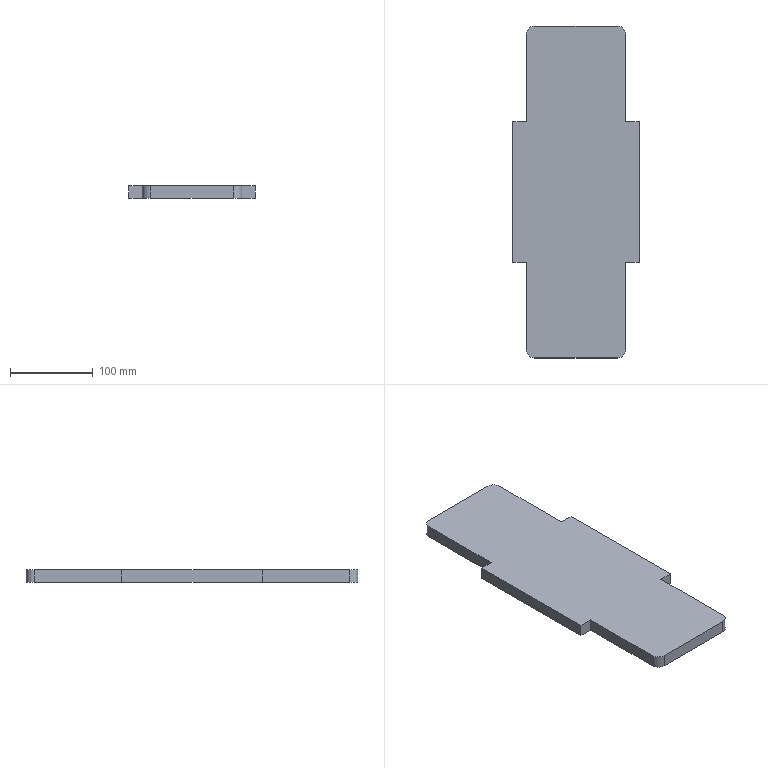Part | STEP file | adapter plate^three-axis module | 1 solid | 18 faces | box 152 x 400 x 15 mm | volume 799832 mm3 | plane 14 | cylinder 4 | commonest cylinder face diameters 20 x4
STEP:
#1=CARTESIAN_POINT('',(-60.,190.,15.));
#2=VERTEX_POINT('',#1);
#3=CARTESIAN_POINT('',(-60.,84.5,15.));
#4=VERTEX_POINT('',#3);
#5=CARTESIAN_POINT('',(-60.,0.,15.));
#6=DIRECTION('',(0.,-1.,0.));
#7=VECTOR('',#6,1000.);
#8=LINE('',#5,#7);
#9=EDGE_CURVE('',#2,#4,#8,.T.);
#10=ORIENTED_EDGE('',*,*,#9,.T.);
#11=CARTESIAN_POINT('',(-76.,84.5,15.));
#12=VERTEX_POINT('',#11);
#13=CARTESIAN_POINT('',(0.,84.5,15.));
#14=DIRECTION('',(-1.,0.,0.));
#15=VECTOR('',#14,1000.);
#16=LINE('',#13,#15);
#17=EDGE_CURVE('',#4,#12,#16,.T.);
#18=ORIENTED_EDGE('',*,*,#17,.T.);
#19=CARTESIAN_POINT('',(-76.,-84.5,15.));
#20=VERTEX_POINT('',#19);
#21=CARTESIAN_POINT('',(-76.,0.,15.));
#22=DIRECTION('',(0.,-1.,0.));
#23=VECTOR('',#22,1000.);
#24=LINE('',#21,#23);
#25=EDGE_CURVE('',#12,#20,#24,.T.);
#26=ORIENTED_EDGE('',*,*,#25,.T.);
#27=CARTESIAN_POINT('',(-60.,-84.5,15.));
#28=VERTEX_POINT('',#27);
#29=CARTESIAN_POINT('',(0.,-84.5,15.));
#30=DIRECTION('',(1.,0.,0.));
#31=VECTOR('',#30,1000.);
#32=LINE('',#29,#31);
#33=EDGE_CURVE('',#20,#28,#32,.T.);
#34=ORIENTED_EDGE('',*,*,#33,.T.);
#35=CARTESIAN_POINT('',(-60.,-190.,15.));
#36=VERTEX_POINT('',#35);
#37=CARTESIAN_POINT('',(-60.,0.,15.));
#38=DIRECTION('',(0.,-1.,0.));
#39=VECTOR('',#38,1000.);
#40=LINE('',#37,#39);
#41=EDGE_CURVE('',#28,#36,#40,.T.);
#42=ORIENTED_EDGE('',*,*,#41,.T.);
#43=CARTESIAN_POINT('',(-50.,-200.,15.));
#44=VERTEX_POINT('',#43);
#45=CARTESIAN_POINT('',(-50.,-190.,15.));
#46=DIRECTION('',(0.,0.,1.));
#47=DIRECTION('',(1.,0.,0.));
#48=AXIS2_PLACEMENT_3D('',#45,#46,#47);
#49=CIRCLE('',#48,10.);
#50=EDGE_CURVE('',#36,#44,#49,.T.);
#51=ORIENTED_EDGE('',*,*,#50,.T.);
#52=CARTESIAN_POINT('',(50.,-200.,15.));
#53=VERTEX_POINT('',#52);
#54=CARTESIAN_POINT('',(0.,-200.,15.));
#55=DIRECTION('',(1.,0.,0.));
#56=VECTOR('',#55,1000.);
#57=LINE('',#54,#56);
#58=EDGE_CURVE('',#44,#53,#57,.T.);
#59=ORIENTED_EDGE('',*,*,#58,.T.);
#60=CARTESIAN_POINT('',(60.,-190.,15.));
#61=VERTEX_POINT('',#60);
#62=CARTESIAN_POINT('',(50.,-190.,15.));
#63=DIRECTION('',(0.,0.,1.));
#64=DIRECTION('',(1.,0.,0.));
#65=AXIS2_PLACEMENT_3D('',#62,#63,#64);
#66=CIRCLE('',#65,10.);
#67=EDGE_CURVE('',#53,#61,#66,.T.);
#68=ORIENTED_EDGE('',*,*,#67,.T.);
#69=CARTESIAN_POINT('',(60.,-84.5,15.));
#70=VERTEX_POINT('',#69);
#71=CARTESIAN_POINT('',(60.,0.,15.));
#72=DIRECTION('',(0.,1.,0.));
#73=VECTOR('',#72,1000.);
#74=LINE('',#71,#73);
#75=EDGE_CURVE('',#61,#70,#74,.T.);
#76=ORIENTED_EDGE('',*,*,#75,.T.);
#77=CARTESIAN_POINT('',(76.,-84.5,15.));
#78=VERTEX_POINT('',#77);
#79=CARTESIAN_POINT('',(0.,-84.5,15.));
#80=DIRECTION('',(1.,0.,0.));
#81=VECTOR('',#80,1000.);
#82=LINE('',#79,#81);
#83=EDGE_CURVE('',#70,#78,#82,.T.);
#84=ORIENTED_EDGE('',*,*,#83,.T.);
#85=CARTESIAN_POINT('',(76.,84.5,15.));
#86=VERTEX_POINT('',#85);
#87=CARTESIAN_POINT('',(76.,0.,15.));
#88=DIRECTION('',(0.,1.,0.));
#89=VECTOR('',#88,1000.);
#90=LINE('',#87,#89);
#91=EDGE_CURVE('',#78,#86,#90,.T.);
#92=ORIENTED_EDGE('',*,*,#91,.T.);
#93=CARTESIAN_POINT('',(60.,84.5,15.));
#94=VERTEX_POINT('',#93);
#95=CARTESIAN_POINT('',(0.,84.5,15.));
#96=DIRECTION('',(-1.,0.,0.));
#97=VECTOR('',#96,1000.);
#98=LINE('',#95,#97);
#99=EDGE_CURVE('',#86,#94,#98,.T.);
#100=ORIENTED_EDGE('',*,*,#99,.T.);
#101=CARTESIAN_POINT('',(60.,190.,15.));
#102=VERTEX_POINT('',#101);
#103=CARTESIAN_POINT('',(60.,0.,15.));
#104=DIRECTION('',(0.,1.,0.));
#105=VECTOR('',#104,1000.);
#106=LINE('',#103,#105);
#107=EDGE_CURVE('',#94,#102,#106,.T.);
#108=ORIENTED_EDGE('',*,*,#107,.T.);
#109=CARTESIAN_POINT('',(50.,200.,15.));
#110=VERTEX_POINT('',#109);
#111=CARTESIAN_POINT('',(50.,190.,15.));
#112=DIRECTION('',(0.,0.,1.));
#113=DIRECTION('',(1.,0.,0.));
#114=AXIS2_PLACEMENT_3D('',#111,#112,#113);
#115=CIRCLE('',#114,10.);
#116=EDGE_CURVE('',#102,#110,#115,.T.);
#117=ORIENTED_EDGE('',*,*,#116,.T.);
#118=CARTESIAN_POINT('',(-50.,200.,15.));
#119=VERTEX_POINT('',#118);
#120=CARTESIAN_POINT('',(0.,200.,15.));
#121=DIRECTION('',(-1.,0.,0.));
#122=VECTOR('',#121,1000.);
#123=LINE('',#120,#122);
#124=EDGE_CURVE('',#110,#119,#123,.T.);
#125=ORIENTED_EDGE('',*,*,#124,.T.);
#126=CARTESIAN_POINT('',(-50.,190.,15.));
#127=DIRECTION('',(0.,0.,1.));
#128=DIRECTION('',(1.,0.,0.));
#129=AXIS2_PLACEMENT_3D('',#126,#127,#128);
#130=CIRCLE('',#129,10.);
#131=EDGE_CURVE('',#119,#2,#130,.T.);
#132=ORIENTED_EDGE('',*,*,#131,.T.);
#133=EDGE_LOOP('',(#10,#18,#26,#34,#42,#51,#59,#68,#76,#84,#92,#100,#108,#117,#125,#132));
#134=FACE_OUTER_BOUND('',#133,.T.);
#135=CARTESIAN_POINT('',(0.,0.,15.));
#136=DIRECTION('',(0.,0.,1.));
#137=DIRECTION('',(1.,0.,0.));
#138=AXIS2_PLACEMENT_3D('',#135,#136,#137);
#139=PLANE('',#138);
#140=ADVANCED_FACE('',(#134),#139,.T.);
#141=CARTESIAN_POINT('',(-76.,84.5,0.));
#142=VERTEX_POINT('',#141);
#143=CARTESIAN_POINT('',(-76.,84.5,15.));
#144=DIRECTION('',(0.,0.,-1.));
#145=VECTOR('',#144,1000.);
#146=LINE('',#143,#145);
#147=EDGE_CURVE('',#12,#142,#146,.T.);
#148=ORIENTED_EDGE('',*,*,#147,.F.);
#149=ORIENTED_EDGE('',*,*,#17,.F.);
#150=CARTESIAN_POINT('',(-60.,84.5,0.));
#151=VERTEX_POINT('',#150);
#152=CARTESIAN_POINT('',(-60.,84.5,15.));
#153=DIRECTION('',(0.,0.,1.));
#154=VECTOR('',#153,1000.);
#155=LINE('',#152,#154);
#156=EDGE_CURVE('',#151,#4,#155,.T.);
#157=ORIENTED_EDGE('',*,*,#156,.F.);
#158=CARTESIAN_POINT('',(-76.,84.5,0.));
#159=DIRECTION('',(1.,0.,0.));
#160=VECTOR('',#159,1000.);
#161=LINE('',#158,#160);
#162=EDGE_CURVE('',#142,#151,#161,.T.);
#163=ORIENTED_EDGE('',*,*,#162,.F.);
#164=EDGE_LOOP('',(#148,#149,#157,#163));
#165=FACE_OUTER_BOUND('',#164,.T.);
#166=CARTESIAN_POINT('',(-76.,84.5,15.));
#167=DIRECTION('',(0.,-1.,0.));
#168=DIRECTION('',(0.,0.,-1.));
#169=AXIS2_PLACEMENT_3D('',#166,#167,#168);
#170=PLANE('',#169);
#171=ADVANCED_FACE('',(#165),#170,.F.);
#172=CARTESIAN_POINT('',(-60.,190.,0.));
#173=VERTEX_POINT('',#172);
#174=CARTESIAN_POINT('',(-60.,200.,0.));
#175=DIRECTION('',(0.,-1.,0.));
#176=VECTOR('',#175,1000.);
#177=LINE('',#174,#176);
#178=EDGE_CURVE('',#173,#151,#177,.T.);
#179=ORIENTED_EDGE('',*,*,#178,.T.);
#180=ORIENTED_EDGE('',*,*,#156,.T.);
#181=ORIENTED_EDGE('',*,*,#9,.F.);
#182=CARTESIAN_POINT('',(-60.,190.,-417.612));
#183=DIRECTION('',(0.,0.,-1.));
#184=VECTOR('',#183,1000.);
#185=LINE('',#182,#184);
#186=EDGE_CURVE('',#2,#173,#185,.T.);
#187=ORIENTED_EDGE('',*,*,#186,.T.);
#188=EDGE_LOOP('',(#179,#180,#181,#187));
#189=FACE_OUTER_BOUND('',#188,.T.);
#190=CARTESIAN_POINT('',(-60.,200.,-417.612));
#191=DIRECTION('',(-1.,0.,0.));
#192=DIRECTION('',(0.,-1.,0.));
#193=AXIS2_PLACEMENT_3D('',#190,#191,#192);
#194=PLANE('',#193);
#195=ADVANCED_FACE('',(#189),#194,.T.);
#196=ORIENTED_EDGE('',*,*,#131,.F.);
#197=CARTESIAN_POINT('',(-50.,200.,0.));
#198=VERTEX_POINT('',#197);
#199=CARTESIAN_POINT('',(-50.,200.,-417.612));
#200=DIRECTION('',(0.,0.,-1.));
#201=VECTOR('',#200,1000.);
#202=LINE('',#199,#201);
#203=EDGE_CURVE('',#119,#198,#202,.T.);
#204=ORIENTED_EDGE('',*,*,#203,.T.);
#205=CARTESIAN_POINT('',(-50.,190.,0.));
#206=DIRECTION('',(0.,0.,1.));
#207=DIRECTION('',(1.,0.,0.));
#208=AXIS2_PLACEMENT_3D('',#205,#206,#207);
#209=CIRCLE('',#208,10.);
#210=EDGE_CURVE('',#198,#173,#209,.T.);
#211=ORIENTED_EDGE('',*,*,#210,.T.);
#212=ORIENTED_EDGE('',*,*,#186,.F.);
#213=EDGE_LOOP('',(#196,#204,#211,#212));
#214=FACE_OUTER_BOUND('',#213,.T.);
#215=CARTESIAN_POINT('',(-50.,190.,-417.612));
#216=DIRECTION('',(0.,0.,1.));
#217=DIRECTION('',(1.,0.,0.));
#218=AXIS2_PLACEMENT_3D('',#215,#216,#217);
#219=CYLINDRICAL_SURFACE('',#218,10.);
#220=ADVANCED_FACE('',(#214),#219,.T.);
#221=CARTESIAN_POINT('',(50.,200.,0.));
#222=VERTEX_POINT('',#221);
#223=CARTESIAN_POINT('',(-60.,200.,0.));
#224=DIRECTION('',(-1.,0.,0.));
#225=VECTOR('',#224,1000.);
#226=LINE('',#223,#225);
#227=EDGE_CURVE('',#222,#198,#226,.T.);
#228=ORIENTED_EDGE('',*,*,#227,.T.);
#229=ORIENTED_EDGE('',*,*,#203,.F.);
#230=ORIENTED_EDGE('',*,*,#124,.F.);
#231=CARTESIAN_POINT('',(50.,200.,-417.612));
#232=DIRECTION('',(0.,0.,-1.));
#233=VECTOR('',#232,1000.);
#234=LINE('',#231,#233);
#235=EDGE_CURVE('',#110,#222,#234,.T.);
#236=ORIENTED_EDGE('',*,*,#235,.T.);
#237=EDGE_LOOP('',(#228,#229,#230,#236));
#238=FACE_OUTER_BOUND('',#237,.T.);
#239=CARTESIAN_POINT('',(-60.,200.,-417.612));
#240=DIRECTION('',(0.,1.,0.));
#241=DIRECTION('',(0.,0.,1.));
#242=AXIS2_PLACEMENT_3D('',#239,#240,#241);
#243=PLANE('',#242);
#244=ADVANCED_FACE('',(#238),#243,.T.);
#245=ORIENTED_EDGE('',*,*,#116,.F.);
#246=CARTESIAN_POINT('',(60.,190.,0.));
#247=VERTEX_POINT('',#246);
#248=CARTESIAN_POINT('',(60.,190.,-417.612));
#249=DIRECTION('',(0.,0.,-1.));
#250=VECTOR('',#249,1000.);
#251=LINE('',#248,#250);
#252=EDGE_CURVE('',#102,#247,#251,.T.);
#253=ORIENTED_EDGE('',*,*,#252,.T.);
#254=CARTESIAN_POINT('',(50.,190.,0.));
#255=DIRECTION('',(0.,0.,1.));
#256=DIRECTION('',(1.,0.,0.));
#257=AXIS2_PLACEMENT_3D('',#254,#255,#256);
#258=CIRCLE('',#257,10.);
#259=EDGE_CURVE('',#247,#222,#258,.T.);
#260=ORIENTED_EDGE('',*,*,#259,.T.);
#261=ORIENTED_EDGE('',*,*,#235,.F.);
#262=EDGE_LOOP('',(#245,#253,#260,#261));
#263=FACE_OUTER_BOUND('',#262,.T.);
#264=CARTESIAN_POINT('',(50.,190.,-417.612));
#265=DIRECTION('',(0.,0.,1.));
#266=DIRECTION('',(1.,0.,0.));
#267=AXIS2_PLACEMENT_3D('',#264,#265,#266);
#268=CYLINDRICAL_SURFACE('',#267,10.);
#269=ADVANCED_FACE('',(#263),#268,.T.);
#270=ORIENTED_EDGE('',*,*,#107,.F.);
#271=CARTESIAN_POINT('',(60.,84.5,0.));
#272=VERTEX_POINT('',#271);
#273=CARTESIAN_POINT('',(60.,84.5,-417.612));
#274=DIRECTION('',(0.,0.,-1.));
#275=VECTOR('',#274,1000.);
#276=LINE('',#273,#275);
#277=EDGE_CURVE('',#94,#272,#276,.T.);
#278=ORIENTED_EDGE('',*,*,#277,.T.);
#279=CARTESIAN_POINT('',(60.,200.,0.));
#280=DIRECTION('',(0.,1.,0.));
#281=VECTOR('',#280,1000.);
#282=LINE('',#279,#281);
#283=EDGE_CURVE('',#272,#247,#282,.T.);
#284=ORIENTED_EDGE('',*,*,#283,.T.);
#285=ORIENTED_EDGE('',*,*,#252,.F.);
#286=EDGE_LOOP('',(#270,#278,#284,#285));
#287=FACE_OUTER_BOUND('',#286,.T.);
#288=CARTESIAN_POINT('',(60.,200.,-417.612));
#289=DIRECTION('',(1.,0.,0.));
#290=DIRECTION('',(0.,1.,0.));
#291=AXIS2_PLACEMENT_3D('',#288,#289,#290);
#292=PLANE('',#291);
#293=ADVANCED_FACE('',(#287),#292,.T.);
#294=CARTESIAN_POINT('',(76.,84.5,0.));
#295=VERTEX_POINT('',#294);
#296=CARTESIAN_POINT('',(76.,84.5,15.));
#297=DIRECTION('',(0.,0.,1.));
#298=VECTOR('',#297,1000.);
#299=LINE('',#296,#298);
#300=EDGE_CURVE('',#295,#86,#299,.T.);
#301=ORIENTED_EDGE('',*,*,#300,.F.);
#302=CARTESIAN_POINT('',(-76.,84.5,0.));
#303=DIRECTION('',(1.,0.,0.));
#304=VECTOR('',#303,1000.);
#305=LINE('',#302,#304);
#306=EDGE_CURVE('',#272,#295,#305,.T.);
#307=ORIENTED_EDGE('',*,*,#306,.F.);
#308=ORIENTED_EDGE('',*,*,#277,.F.);
#309=ORIENTED_EDGE('',*,*,#99,.F.);
#310=EDGE_LOOP('',(#301,#307,#308,#309));
#311=FACE_OUTER_BOUND('',#310,.T.);
#312=CARTESIAN_POINT('',(-76.,84.5,15.));
#313=DIRECTION('',(0.,-1.,0.));
#314=DIRECTION('',(0.,0.,-1.));
#315=AXIS2_PLACEMENT_3D('',#312,#313,#314);
#316=PLANE('',#315);
#317=ADVANCED_FACE('',(#311),#316,.F.);
#318=CARTESIAN_POINT('',(76.,-84.5,0.));
#319=VERTEX_POINT('',#318);
#320=CARTESIAN_POINT('',(76.,-84.5,15.));
#321=DIRECTION('',(0.,0.,1.));
#322=VECTOR('',#321,1000.);
#323=LINE('',#320,#322);
#324=EDGE_CURVE('',#319,#78,#323,.T.);
#325=ORIENTED_EDGE('',*,*,#324,.F.);
#326=CARTESIAN_POINT('',(76.,84.5,0.));
#327=DIRECTION('',(0.,-1.,0.));
#328=VECTOR('',#327,1000.);
#329=LINE('',#326,#328);
#330=EDGE_CURVE('',#295,#319,#329,.T.);
#331=ORIENTED_EDGE('',*,*,#330,.F.);
#332=ORIENTED_EDGE('',*,*,#300,.T.);
#333=ORIENTED_EDGE('',*,*,#91,.F.);
#334=EDGE_LOOP('',(#325,#331,#332,#333));
#335=FACE_OUTER_BOUND('',#334,.T.);
#336=CARTESIAN_POINT('',(76.,84.5,15.));
#337=DIRECTION('',(-1.,0.,0.));
#338=DIRECTION('',(0.,0.,1.));
#339=AXIS2_PLACEMENT_3D('',#336,#337,#338);
#340=PLANE('',#339);
#341=ADVANCED_FACE('',(#335),#340,.F.);
#342=ORIENTED_EDGE('',*,*,#324,.T.);
#343=ORIENTED_EDGE('',*,*,#83,.F.);
#344=CARTESIAN_POINT('',(60.,-84.5,0.));
#345=VERTEX_POINT('',#344);
#346=CARTESIAN_POINT('',(60.,-84.5,15.));
#347=DIRECTION('',(0.,0.,1.));
#348=VECTOR('',#347,1000.);
#349=LINE('',#346,#348);
#350=EDGE_CURVE('',#345,#70,#349,.T.);
#351=ORIENTED_EDGE('',*,*,#350,.F.);
#352=CARTESIAN_POINT('',(-76.,-84.5,0.));
#353=DIRECTION('',(-1.,0.,0.));
#354=VECTOR('',#353,1000.);
#355=LINE('',#352,#354);
#356=EDGE_CURVE('',#319,#345,#355,.T.);
#357=ORIENTED_EDGE('',*,*,#356,.F.);
#358=EDGE_LOOP('',(#342,#343,#351,#357));
#359=FACE_OUTER_BOUND('',#358,.T.);
#360=CARTESIAN_POINT('',(-76.,-84.5,15.));
#361=DIRECTION('',(0.,1.,0.));
#362=DIRECTION('',(0.,0.,1.));
#363=AXIS2_PLACEMENT_3D('',#360,#361,#362);
#364=PLANE('',#363);
#365=ADVANCED_FACE('',(#359),#364,.F.);
#366=CARTESIAN_POINT('',(60.,-190.,0.));
#367=VERTEX_POINT('',#366);
#368=CARTESIAN_POINT('',(60.,200.,0.));
#369=DIRECTION('',(0.,1.,0.));
#370=VECTOR('',#369,1000.);
#371=LINE('',#368,#370);
#372=EDGE_CURVE('',#367,#345,#371,.T.);
#373=ORIENTED_EDGE('',*,*,#372,.T.);
#374=ORIENTED_EDGE('',*,*,#350,.T.);
#375=ORIENTED_EDGE('',*,*,#75,.F.);
#376=CARTESIAN_POINT('',(60.,-190.,-417.612));
#377=DIRECTION('',(0.,0.,-1.));
#378=VECTOR('',#377,1000.);
#379=LINE('',#376,#378);
#380=EDGE_CURVE('',#61,#367,#379,.T.);
#381=ORIENTED_EDGE('',*,*,#380,.T.);
#382=EDGE_LOOP('',(#373,#374,#375,#381));
#383=FACE_OUTER_BOUND('',#382,.T.);
#384=CARTESIAN_POINT('',(60.,200.,-417.612));
#385=DIRECTION('',(1.,0.,0.));
#386=DIRECTION('',(0.,1.,0.));
#387=AXIS2_PLACEMENT_3D('',#384,#385,#386);
#388=PLANE('',#387);
#389=ADVANCED_FACE('',(#383),#388,.T.);
#390=ORIENTED_EDGE('',*,*,#67,.F.);
#391=CARTESIAN_POINT('',(50.,-200.,0.));
#392=VERTEX_POINT('',#391);
#393=CARTESIAN_POINT('',(50.,-200.,-417.612));
#394=DIRECTION('',(0.,0.,-1.));
#395=VECTOR('',#394,1000.);
#396=LINE('',#393,#395);
#397=EDGE_CURVE('',#53,#392,#396,.T.);
#398=ORIENTED_EDGE('',*,*,#397,.T.);
#399=CARTESIAN_POINT('',(50.,-190.,0.));
#400=DIRECTION('',(0.,0.,1.));
#401=DIRECTION('',(1.,0.,0.));
#402=AXIS2_PLACEMENT_3D('',#399,#400,#401);
#403=CIRCLE('',#402,10.);
#404=EDGE_CURVE('',#392,#367,#403,.T.);
#405=ORIENTED_EDGE('',*,*,#404,.T.);
#406=ORIENTED_EDGE('',*,*,#380,.F.);
#407=EDGE_LOOP('',(#390,#398,#405,#406));
#408=FACE_OUTER_BOUND('',#407,.T.);
#409=CARTESIAN_POINT('',(50.,-190.,-417.612));
#410=DIRECTION('',(0.,0.,1.));
#411=DIRECTION('',(1.,0.,0.));
#412=AXIS2_PLACEMENT_3D('',#409,#410,#411);
#413=CYLINDRICAL_SURFACE('',#412,10.);
#414=ADVANCED_FACE('',(#408),#413,.T.);
#415=ORIENTED_EDGE('',*,*,#58,.F.);
#416=CARTESIAN_POINT('',(-50.,-200.,0.));
#417=VERTEX_POINT('',#416);
#418=CARTESIAN_POINT('',(-50.,-200.,-417.612));
#419=DIRECTION('',(0.,0.,-1.));
#420=VECTOR('',#419,1000.);
#421=LINE('',#418,#420);
#422=EDGE_CURVE('',#44,#417,#421,.T.);
#423=ORIENTED_EDGE('',*,*,#422,.T.);
#424=CARTESIAN_POINT('',(-60.,-200.,0.));
#425=DIRECTION('',(1.,0.,0.));
#426=VECTOR('',#425,1000.);
#427=LINE('',#424,#426);
#428=EDGE_CURVE('',#417,#392,#427,.T.);
#429=ORIENTED_EDGE('',*,*,#428,.T.);
#430=ORIENTED_EDGE('',*,*,#397,.F.);
#431=EDGE_LOOP('',(#415,#423,#429,#430));
#432=FACE_OUTER_BOUND('',#431,.T.);
#433=CARTESIAN_POINT('',(-60.,-200.,-417.612));
#434=DIRECTION('',(0.,-1.,0.));
#435=DIRECTION('',(0.,0.,-1.));
#436=AXIS2_PLACEMENT_3D('',#433,#434,#435);
#437=PLANE('',#436);
#438=ADVANCED_FACE('',(#432),#437,.T.);
#439=ORIENTED_EDGE('',*,*,#50,.F.);
#440=CARTESIAN_POINT('',(-60.,-190.,0.));
#441=VERTEX_POINT('',#440);
#442=CARTESIAN_POINT('',(-60.,-190.,-417.612));
#443=DIRECTION('',(0.,0.,-1.));
#444=VECTOR('',#443,1000.);
#445=LINE('',#442,#444);
#446=EDGE_CURVE('',#36,#441,#445,.T.);
#447=ORIENTED_EDGE('',*,*,#446,.T.);
#448=CARTESIAN_POINT('',(-50.,-190.,0.));
#449=DIRECTION('',(0.,0.,1.));
#450=DIRECTION('',(1.,0.,0.));
#451=AXIS2_PLACEMENT_3D('',#448,#449,#450);
#452=CIRCLE('',#451,10.);
#453=EDGE_CURVE('',#441,#417,#452,.T.);
#454=ORIENTED_EDGE('',*,*,#453,.T.);
#455=ORIENTED_EDGE('',*,*,#422,.F.);
#456=EDGE_LOOP('',(#439,#447,#454,#455));
#457=FACE_OUTER_BOUND('',#456,.T.);
#458=CARTESIAN_POINT('',(-50.,-190.,-417.612));
#459=DIRECTION('',(0.,0.,1.));
#460=DIRECTION('',(1.,0.,0.));
#461=AXIS2_PLACEMENT_3D('',#458,#459,#460);
#462=CYLINDRICAL_SURFACE('',#461,10.);
#463=ADVANCED_FACE('',(#457),#462,.T.);
#464=ORIENTED_EDGE('',*,*,#41,.F.);
#465=CARTESIAN_POINT('',(-60.,-84.5,0.));
#466=VERTEX_POINT('',#465);
#467=CARTESIAN_POINT('',(-60.,-84.5,-417.612));
#468=DIRECTION('',(0.,0.,-1.));
#469=VECTOR('',#468,1000.);
#470=LINE('',#467,#469);
#471=EDGE_CURVE('',#28,#466,#470,.T.);
#472=ORIENTED_EDGE('',*,*,#471,.T.);
#473=CARTESIAN_POINT('',(-60.,200.,0.));
#474=DIRECTION('',(0.,-1.,0.));
#475=VECTOR('',#474,1000.);
#476=LINE('',#473,#475);
#477=EDGE_CURVE('',#466,#441,#476,.T.);
#478=ORIENTED_EDGE('',*,*,#477,.T.);
#479=ORIENTED_EDGE('',*,*,#446,.F.);
#480=EDGE_LOOP('',(#464,#472,#478,#479));
#481=FACE_OUTER_BOUND('',#480,.T.);
#482=CARTESIAN_POINT('',(-60.,200.,-417.612));
#483=DIRECTION('',(-1.,0.,0.));
#484=DIRECTION('',(0.,-1.,0.));
#485=AXIS2_PLACEMENT_3D('',#482,#483,#484);
#486=PLANE('',#485);
#487=ADVANCED_FACE('',(#481),#486,.T.);
#488=CARTESIAN_POINT('',(-76.,-84.5,0.));
#489=VERTEX_POINT('',#488);
#490=CARTESIAN_POINT('',(-76.,-84.5,15.));
#491=DIRECTION('',(0.,0.,1.));
#492=VECTOR('',#491,1000.);
#493=LINE('',#490,#492);
#494=EDGE_CURVE('',#489,#20,#493,.T.);
#495=ORIENTED_EDGE('',*,*,#494,.F.);
#496=CARTESIAN_POINT('',(-76.,-84.5,0.));
#497=DIRECTION('',(-1.,0.,0.));
#498=VECTOR('',#497,1000.);
#499=LINE('',#496,#498);
#500=EDGE_CURVE('',#466,#489,#499,.T.);
#501=ORIENTED_EDGE('',*,*,#500,.F.);
#502=ORIENTED_EDGE('',*,*,#471,.F.);
#503=ORIENTED_EDGE('',*,*,#33,.F.);
#504=EDGE_LOOP('',(#495,#501,#502,#503));
#505=FACE_OUTER_BOUND('',#504,.T.);
#506=CARTESIAN_POINT('',(-76.,-84.5,15.));
#507=DIRECTION('',(0.,1.,0.));
#508=DIRECTION('',(0.,0.,1.));
#509=AXIS2_PLACEMENT_3D('',#506,#507,#508);
#510=PLANE('',#509);
#511=ADVANCED_FACE('',(#505),#510,.F.);
#512=ORIENTED_EDGE('',*,*,#147,.T.);
#513=CARTESIAN_POINT('',(-76.,84.5,0.));
#514=DIRECTION('',(0.,1.,0.));
#515=VECTOR('',#514,1000.);
#516=LINE('',#513,#515);
#517=EDGE_CURVE('',#489,#142,#516,.T.);
#518=ORIENTED_EDGE('',*,*,#517,.F.);
#519=ORIENTED_EDGE('',*,*,#494,.T.);
#520=ORIENTED_EDGE('',*,*,#25,.F.);
#521=EDGE_LOOP('',(#512,#518,#519,#520));
#522=FACE_OUTER_BOUND('',#521,.T.);
#523=CARTESIAN_POINT('',(-76.,84.5,15.));
#524=DIRECTION('',(1.,0.,0.));
#525=DIRECTION('',(0.,1.,0.));
#526=AXIS2_PLACEMENT_3D('',#523,#524,#525);
#527=PLANE('',#526);
#528=ADVANCED_FACE('',(#522),#527,.F.);
#529=ORIENTED_EDGE('',*,*,#453,.F.);
#530=ORIENTED_EDGE('',*,*,#477,.F.);
#531=ORIENTED_EDGE('',*,*,#500,.T.);
#532=ORIENTED_EDGE('',*,*,#517,.T.);
#533=ORIENTED_EDGE('',*,*,#162,.T.);
#534=ORIENTED_EDGE('',*,*,#178,.F.);
#535=ORIENTED_EDGE('',*,*,#210,.F.);
#536=ORIENTED_EDGE('',*,*,#227,.F.);
#537=ORIENTED_EDGE('',*,*,#259,.F.);
#538=ORIENTED_EDGE('',*,*,#283,.F.);
#539=ORIENTED_EDGE('',*,*,#306,.T.);
#540=ORIENTED_EDGE('',*,*,#330,.T.);
#541=ORIENTED_EDGE('',*,*,#356,.T.);
#542=ORIENTED_EDGE('',*,*,#372,.F.);
#543=ORIENTED_EDGE('',*,*,#404,.F.);
#544=ORIENTED_EDGE('',*,*,#428,.F.);
#545=EDGE_LOOP('',(#529,#530,#531,#532,#533,#534,#535,#536,#537,#538,#539,#540,#541,#542,#543,#544));
#546=FACE_OUTER_BOUND('',#545,.T.);
#547=CARTESIAN_POINT('',(0.,0.,0.));
#548=DIRECTION('',(0.,0.,1.));
#549=DIRECTION('',(1.,0.,0.));
#550=AXIS2_PLACEMENT_3D('',#547,#548,#549);
#551=PLANE('',#550);
#552=ADVANCED_FACE('',(#546),#551,.F.);
#553=CLOSED_SHELL('',(#140,#171,#195,#220,#244,#269,#293,#317,#341,#365,#389,#414,#438,#463,#487,#511,#528,#552));
#554=MANIFOLD_SOLID_BREP('',#553);
#555=CARTESIAN_POINT('',(0.,0.,0.));
#556=DIRECTION('',(0.,0.,1.));
#557=DIRECTION('',(1.,0.,0.));
#558=AXIS2_PLACEMENT_3D('',#555,#556,#557);
#559=(LENGTH_UNIT()NAMED_UNIT(*)SI_UNIT(.MILLI.,.METRE.));
#560=UNCERTAINTY_MEASURE_WITH_UNIT(LENGTH_MEASURE(0.00001),#559,'','');
#561=(NAMED_UNIT(*)PLANE_ANGLE_UNIT()SI_UNIT($,.RADIAN.));
#562=(NAMED_UNIT(*)SI_UNIT($,.STERADIAN.)SOLID_ANGLE_UNIT());
#563=(GEOMETRIC_REPRESENTATION_CONTEXT(3)GLOBAL_UNCERTAINTY_ASSIGNED_CONTEXT((#560))GLOBAL_UNIT_ASSIGNED_CONTEXT((#559,#561,#562))REPRESENTATION_CONTEXT('',''));
#564=ADVANCED_BREP_SHAPE_REPRESENTATION('',(#554,#558),#563);